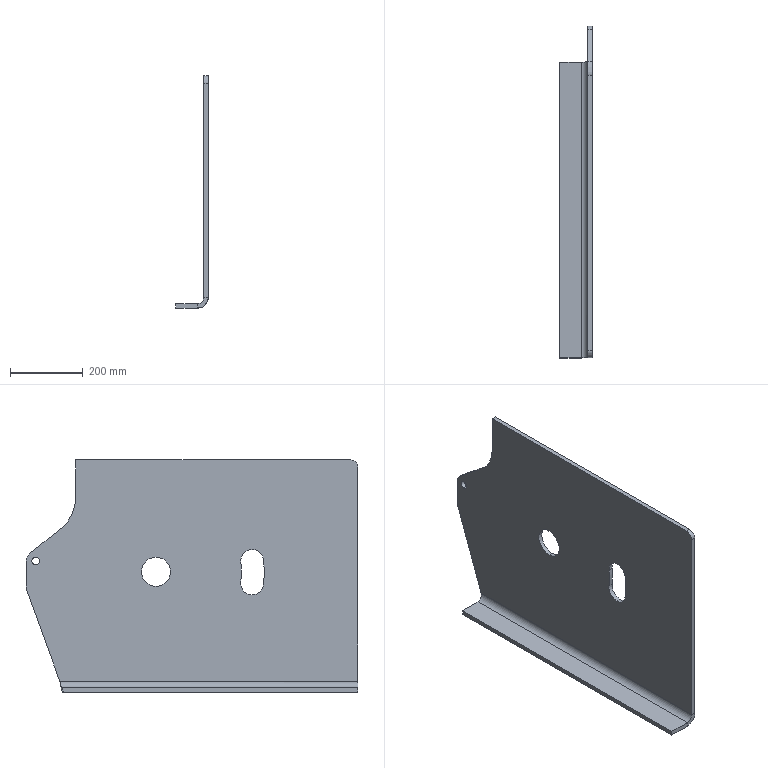Part | SolidWorks | features DeleteBody 1, FlatPattern 1, MBimport 1, SheetMetal 1, SolidToSheetMetal 1 | 2 solids | 56 faces | box 89 x 910.92 x 637.5 mm | volume 13906050 mm3 | cylinder 30 | plane 25 | spline 1 | commonest cylinder face diameters 62.6 x6 20.686 x4 36 x4 80 x4 40 x2 52 x2